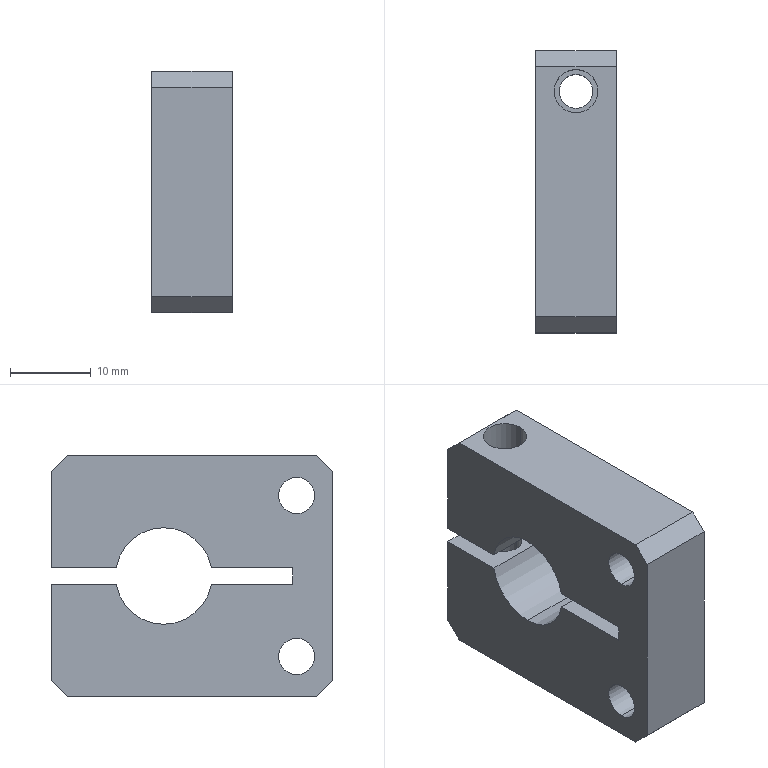Part | STEP file | 11-FG-S02211 | 1 solid | 33 faces | box 10 x 35 x 30 mm | volume 7793 mm3 | plane 18 | cylinder 15 | commonest cylinder face diameters 4.5 x4 8 x4 12 x3 4.2 x2 5.4 x2
STEP:
#1=CARTESIAN_POINT('',(0.6,-13.,-6.));
#2=VERTEX_POINT('',#1);
#3=CARTESIAN_POINT('',(0.6,-13.,-14.));
#4=VERTEX_POINT('',#3);
#5=CARTESIAN_POINT('',(0.6,-13.,-10.));
#6=DIRECTION('',(1.,0.,0.));
#7=DIRECTION('',(0.,0.,-1.));
#8=AXIS2_PLACEMENT_3D('',#5,#6,#7);
#9=CIRCLE('',#8,4.);
#10=EDGE_CURVE('',#2,#4,#9,.T.);
#11=ORIENTED_EDGE('',*,*,#10,.F.);
#12=CARTESIAN_POINT('',(5.,-13.,-6.));
#13=VERTEX_POINT('',#12);
#14=CARTESIAN_POINT('',(5.,-13.,-6.));
#15=DIRECTION('',(1.,0.,0.));
#16=VECTOR('',#15,1000.);
#17=LINE('',#14,#16);
#18=EDGE_CURVE('',#2,#13,#17,.T.);
#19=ORIENTED_EDGE('',*,*,#18,.T.);
#20=CARTESIAN_POINT('',(5.,-13.,-14.));
#21=VERTEX_POINT('',#20);
#22=CARTESIAN_POINT('',(5.,-13.,-10.));
#23=DIRECTION('',(1.,0.,0.));
#24=DIRECTION('',(0.,0.,-1.));
#25=AXIS2_PLACEMENT_3D('',#22,#23,#24);
#26=CIRCLE('',#25,4.);
#27=EDGE_CURVE('',#13,#21,#26,.T.);
#28=ORIENTED_EDGE('',*,*,#27,.T.);
#29=CARTESIAN_POINT('',(5.,-13.,-14.));
#30=DIRECTION('',(1.,0.,0.));
#31=VECTOR('',#30,1000.);
#32=LINE('',#29,#31);
#33=EDGE_CURVE('',#4,#21,#32,.T.);
#34=ORIENTED_EDGE('',*,*,#33,.F.);
#35=EDGE_LOOP('',(#11,#19,#28,#34));
#36=FACE_OUTER_BOUND('',#35,.T.);
#37=CARTESIAN_POINT('',(5.,-13.,-10.));
#38=DIRECTION('',(1.,0.,0.));
#39=DIRECTION('',(0.,0.,-1.));
#40=AXIS2_PLACEMENT_3D('',#37,#38,#39);
#41=CYLINDRICAL_SURFACE('',#40,4.);
#42=ADVANCED_FACE('',(#36),#41,.F.);
#43=CARTESIAN_POINT('',(-5.,-13.,-7.75));
#44=VERTEX_POINT('',#43);
#45=CARTESIAN_POINT('',(-5.,-13.,-12.25));
#46=VERTEX_POINT('',#45);
#47=CARTESIAN_POINT('',(-5.,-13.,-10.));
#48=DIRECTION('',(1.,0.,0.));
#49=DIRECTION('',(0.,0.,-1.));
#50=AXIS2_PLACEMENT_3D('',#47,#48,#49);
#51=CIRCLE('',#50,2.25);
#52=EDGE_CURVE('',#44,#46,#51,.T.);
#53=ORIENTED_EDGE('',*,*,#52,.F.);
#54=CARTESIAN_POINT('',(0.6,-13.,-7.75));
#55=VERTEX_POINT('',#54);
#56=CARTESIAN_POINT('',(5.,-13.,-7.75));
#57=DIRECTION('',(1.,0.,0.));
#58=VECTOR('',#57,1000.);
#59=LINE('',#56,#58);
#60=EDGE_CURVE('',#44,#55,#59,.T.);
#61=ORIENTED_EDGE('',*,*,#60,.T.);
#62=CARTESIAN_POINT('',(0.6,-13.,-12.25));
#63=VERTEX_POINT('',#62);
#64=CARTESIAN_POINT('',(0.6,-13.,-10.));
#65=DIRECTION('',(1.,0.,0.));
#66=DIRECTION('',(0.,0.,-1.));
#67=AXIS2_PLACEMENT_3D('',#64,#65,#66);
#68=CIRCLE('',#67,2.25);
#69=EDGE_CURVE('',#55,#63,#68,.T.);
#70=ORIENTED_EDGE('',*,*,#69,.T.);
#71=CARTESIAN_POINT('',(5.,-13.,-12.25));
#72=DIRECTION('',(1.,0.,0.));
#73=VECTOR('',#72,1000.);
#74=LINE('',#71,#73);
#75=EDGE_CURVE('',#46,#63,#74,.T.);
#76=ORIENTED_EDGE('',*,*,#75,.F.);
#77=EDGE_LOOP('',(#53,#61,#70,#76));
#78=FACE_OUTER_BOUND('',#77,.T.);
#79=CARTESIAN_POINT('',(5.,-13.,-10.));
#80=DIRECTION('',(1.,0.,0.));
#81=DIRECTION('',(0.,0.,-1.));
#82=AXIS2_PLACEMENT_3D('',#79,#80,#81);
#83=CYLINDRICAL_SURFACE('',#82,2.25);
#84=ADVANCED_FACE('',(#78),#83,.F.);
#85=CARTESIAN_POINT('',(0.6,-13.,14.));
#86=VERTEX_POINT('',#85);
#87=CARTESIAN_POINT('',(0.6,-13.,6.));
#88=VERTEX_POINT('',#87);
#89=CARTESIAN_POINT('',(0.6,-13.,10.));
#90=DIRECTION('',(1.,0.,0.));
#91=DIRECTION('',(0.,0.,-1.));
#92=AXIS2_PLACEMENT_3D('',#89,#90,#91);
#93=CIRCLE('',#92,4.);
#94=EDGE_CURVE('',#86,#88,#93,.T.);
#95=ORIENTED_EDGE('',*,*,#94,.F.);
#96=CARTESIAN_POINT('',(5.,-13.,14.));
#97=VERTEX_POINT('',#96);
#98=CARTESIAN_POINT('',(5.,-13.,14.));
#99=DIRECTION('',(1.,0.,0.));
#100=VECTOR('',#99,1000.);
#101=LINE('',#98,#100);
#102=EDGE_CURVE('',#86,#97,#101,.T.);
#103=ORIENTED_EDGE('',*,*,#102,.T.);
#104=CARTESIAN_POINT('',(5.,-13.,6.));
#105=VERTEX_POINT('',#104);
#106=CARTESIAN_POINT('',(5.,-13.,10.));
#107=DIRECTION('',(1.,0.,0.));
#108=DIRECTION('',(0.,0.,-1.));
#109=AXIS2_PLACEMENT_3D('',#106,#107,#108);
#110=CIRCLE('',#109,4.);
#111=EDGE_CURVE('',#97,#105,#110,.T.);
#112=ORIENTED_EDGE('',*,*,#111,.T.);
#113=CARTESIAN_POINT('',(5.,-13.,6.));
#114=DIRECTION('',(1.,0.,0.));
#115=VECTOR('',#114,1000.);
#116=LINE('',#113,#115);
#117=EDGE_CURVE('',#88,#105,#116,.T.);
#118=ORIENTED_EDGE('',*,*,#117,.F.);
#119=EDGE_LOOP('',(#95,#103,#112,#118));
#120=FACE_OUTER_BOUND('',#119,.T.);
#121=CARTESIAN_POINT('',(5.,-13.,10.));
#122=DIRECTION('',(1.,0.,0.));
#123=DIRECTION('',(0.,0.,-1.));
#124=AXIS2_PLACEMENT_3D('',#121,#122,#123);
#125=CYLINDRICAL_SURFACE('',#124,4.);
#126=ADVANCED_FACE('',(#120),#125,.F.);
#127=CARTESIAN_POINT('',(-5.,-13.,12.25));
#128=VERTEX_POINT('',#127);
#129=CARTESIAN_POINT('',(-5.,-13.,7.75));
#130=VERTEX_POINT('',#129);
#131=CARTESIAN_POINT('',(-5.,-13.,10.));
#132=DIRECTION('',(1.,0.,0.));
#133=DIRECTION('',(0.,0.,-1.));
#134=AXIS2_PLACEMENT_3D('',#131,#132,#133);
#135=CIRCLE('',#134,2.25);
#136=EDGE_CURVE('',#128,#130,#135,.T.);
#137=ORIENTED_EDGE('',*,*,#136,.F.);
#138=CARTESIAN_POINT('',(0.6,-13.,12.25));
#139=VERTEX_POINT('',#138);
#140=CARTESIAN_POINT('',(5.,-13.,12.25));
#141=DIRECTION('',(1.,0.,0.));
#142=VECTOR('',#141,1000.);
#143=LINE('',#140,#142);
#144=EDGE_CURVE('',#128,#139,#143,.T.);
#145=ORIENTED_EDGE('',*,*,#144,.T.);
#146=CARTESIAN_POINT('',(0.6,-13.,7.75));
#147=VERTEX_POINT('',#146);
#148=CARTESIAN_POINT('',(0.6,-13.,10.));
#149=DIRECTION('',(1.,0.,0.));
#150=DIRECTION('',(0.,0.,-1.));
#151=AXIS2_PLACEMENT_3D('',#148,#149,#150);
#152=CIRCLE('',#151,2.25);
#153=EDGE_CURVE('',#139,#147,#152,.T.);
#154=ORIENTED_EDGE('',*,*,#153,.T.);
#155=CARTESIAN_POINT('',(5.,-13.,7.75));
#156=DIRECTION('',(1.,0.,0.));
#157=VECTOR('',#156,1000.);
#158=LINE('',#155,#157);
#159=EDGE_CURVE('',#130,#147,#158,.T.);
#160=ORIENTED_EDGE('',*,*,#159,.F.);
#161=EDGE_LOOP('',(#137,#145,#154,#160));
#162=FACE_OUTER_BOUND('',#161,.T.);
#163=CARTESIAN_POINT('',(5.,-13.,10.));
#164=DIRECTION('',(1.,0.,0.));
#165=DIRECTION('',(0.,0.,-1.));
#166=AXIS2_PLACEMENT_3D('',#163,#164,#165);
#167=CYLINDRICAL_SURFACE('',#166,2.25);
#168=ADVANCED_FACE('',(#162),#167,.F.);
#169=CARTESIAN_POINT('',(2.1,12.5,-15.));
#170=VERTEX_POINT('',#169);
#171=CARTESIAN_POINT('',(-2.1,12.5,-15.));
#172=VERTEX_POINT('',#171);
#173=CARTESIAN_POINT('',(0.,12.5,-15.));
#174=DIRECTION('',(0.,0.,-1.));
#175=DIRECTION('',(-1.,0.,0.));
#176=AXIS2_PLACEMENT_3D('',#173,#174,#175);
#177=CIRCLE('',#176,2.1);
#178=EDGE_CURVE('',#170,#172,#177,.T.);
#179=ORIENTED_EDGE('',*,*,#178,.T.);
#180=CARTESIAN_POINT('',(-2.1,12.5,-1.));
#181=VERTEX_POINT('',#180);
#182=CARTESIAN_POINT('',(-2.1,12.5,-1.));
#183=DIRECTION('',(0.,0.,1.));
#184=VECTOR('',#183,1000.);
#185=LINE('',#182,#184);
#186=EDGE_CURVE('',#172,#181,#185,.T.);
#187=ORIENTED_EDGE('',*,*,#186,.T.);
#188=CARTESIAN_POINT('',(2.1,12.5,-1.));
#189=VERTEX_POINT('',#188);
#190=CARTESIAN_POINT('',(0.,12.5,-1.));
#191=DIRECTION('',(0.,0.,1.));
#192=DIRECTION('',(1.,0.,0.));
#193=AXIS2_PLACEMENT_3D('',#190,#191,#192);
#194=CIRCLE('',#193,2.1);
#195=EDGE_CURVE('',#181,#189,#194,.T.);
#196=ORIENTED_EDGE('',*,*,#195,.T.);
#197=CARTESIAN_POINT('',(2.1,12.5,-1.));
#198=DIRECTION('',(0.,0.,1.));
#199=VECTOR('',#198,1000.);
#200=LINE('',#197,#199);
#201=EDGE_CURVE('',#170,#189,#200,.T.);
#202=ORIENTED_EDGE('',*,*,#201,.F.);
#203=EDGE_LOOP('',(#179,#187,#196,#202));
#204=FACE_OUTER_BOUND('',#203,.T.);
#205=CARTESIAN_POINT('',(0.,12.5,-1.));
#206=DIRECTION('',(0.,0.,1.));
#207=DIRECTION('',(1.,0.,0.));
#208=AXIS2_PLACEMENT_3D('',#205,#206,#207);
#209=CYLINDRICAL_SURFACE('',#208,2.1);
#210=ADVANCED_FACE('',(#204),#209,.F.);
#211=CARTESIAN_POINT('',(-2.7,12.5,1.));
#212=VERTEX_POINT('',#211);
#213=CARTESIAN_POINT('',(2.7,12.5,1.));
#214=VERTEX_POINT('',#213);
#215=CARTESIAN_POINT('',(0.,12.5,1.));
#216=DIRECTION('',(0.,0.,1.));
#217=DIRECTION('',(0.,-1.,0.));
#218=AXIS2_PLACEMENT_3D('',#215,#216,#217);
#219=CIRCLE('',#218,2.7);
#220=EDGE_CURVE('',#212,#214,#219,.T.);
#221=ORIENTED_EDGE('',*,*,#220,.F.);
#222=CARTESIAN_POINT('',(-2.7,12.5,15.));
#223=VERTEX_POINT('',#222);
#224=CARTESIAN_POINT('',(-2.7,12.5,15.));
#225=DIRECTION('',(0.,0.,1.));
#226=VECTOR('',#225,1000.);
#227=LINE('',#224,#226);
#228=EDGE_CURVE('',#212,#223,#227,.T.);
#229=ORIENTED_EDGE('',*,*,#228,.T.);
#230=CARTESIAN_POINT('',(2.7,12.5,15.));
#231=VERTEX_POINT('',#230);
#232=CARTESIAN_POINT('',(0.,12.5,15.));
#233=DIRECTION('',(0.,0.,1.));
#234=DIRECTION('',(1.,0.,0.));
#235=AXIS2_PLACEMENT_3D('',#232,#233,#234);
#236=CIRCLE('',#235,2.7);
#237=EDGE_CURVE('',#223,#231,#236,.T.);
#238=ORIENTED_EDGE('',*,*,#237,.T.);
#239=CARTESIAN_POINT('',(2.7,12.5,15.));
#240=DIRECTION('',(0.,0.,1.));
#241=VECTOR('',#240,1000.);
#242=LINE('',#239,#241);
#243=EDGE_CURVE('',#214,#231,#242,.T.);
#244=ORIENTED_EDGE('',*,*,#243,.F.);
#245=EDGE_LOOP('',(#221,#229,#238,#244));
#246=FACE_OUTER_BOUND('',#245,.T.);
#247=CARTESIAN_POINT('',(0.,12.5,15.));
#248=DIRECTION('',(0.,0.,1.));
#249=DIRECTION('',(1.,0.,0.));
#250=AXIS2_PLACEMENT_3D('',#247,#248,#249);
#251=CYLINDRICAL_SURFACE('',#250,2.7);
#252=ADVANCED_FACE('',(#246),#251,.F.);
#253=CARTESIAN_POINT('',(-5.,3.5,-6.));
#254=VERTEX_POINT('',#253);
#255=CARTESIAN_POINT('',(-5.,9.416,-1.));
#256=VERTEX_POINT('',#255);
#257=CARTESIAN_POINT('',(-5.,3.5,0.));
#258=DIRECTION('',(1.,0.,0.));
#259=DIRECTION('',(0.,0.,-1.));
#260=AXIS2_PLACEMENT_3D('',#257,#258,#259);
#261=CIRCLE('',#260,6.);
#262=EDGE_CURVE('',#254,#256,#261,.T.);
#263=ORIENTED_EDGE('',*,*,#262,.F.);
#264=CARTESIAN_POINT('',(5.,3.5,-6.));
#265=VERTEX_POINT('',#264);
#266=CARTESIAN_POINT('',(-5.,3.5,-6.));
#267=DIRECTION('',(1.,0.,0.));
#268=VECTOR('',#267,1000.);
#269=LINE('',#266,#268);
#270=EDGE_CURVE('',#254,#265,#269,.T.);
#271=ORIENTED_EDGE('',*,*,#270,.T.);
#272=CARTESIAN_POINT('',(5.,9.416,-1.));
#273=VERTEX_POINT('',#272);
#274=CARTESIAN_POINT('',(5.,3.5,0.));
#275=DIRECTION('',(1.,0.,0.));
#276=DIRECTION('',(0.,0.,-1.));
#277=AXIS2_PLACEMENT_3D('',#274,#275,#276);
#278=CIRCLE('',#277,6.);
#279=EDGE_CURVE('',#265,#273,#278,.T.);
#280=ORIENTED_EDGE('',*,*,#279,.T.);
#281=CARTESIAN_POINT('',(-5.,9.416,-1.));
#282=DIRECTION('',(-1.,0.,0.));
#283=VECTOR('',#282,1000.);
#284=LINE('',#281,#283);
#285=EDGE_CURVE('',#273,#256,#284,.T.);
#286=ORIENTED_EDGE('',*,*,#285,.T.);
#287=EDGE_LOOP('',(#263,#271,#280,#286));
#288=FACE_OUTER_BOUND('',#287,.T.);
#289=CARTESIAN_POINT('',(-5.,3.5,0.));
#290=DIRECTION('',(1.,0.,0.));
#291=DIRECTION('',(0.,0.,-1.));
#292=AXIS2_PLACEMENT_3D('',#289,#290,#291);
#293=CYLINDRICAL_SURFACE('',#292,6.);
#294=ADVANCED_FACE('',(#288),#293,.F.);
#295=CARTESIAN_POINT('',(5.,17.5,-1.));
#296=VERTEX_POINT('',#295);
#297=CARTESIAN_POINT('',(5.,17.5,-1.));
#298=DIRECTION('',(0.,1.,0.));
#299=VECTOR('',#298,1000.);
#300=LINE('',#297,#299);
#301=EDGE_CURVE('',#273,#296,#300,.T.);
#302=ORIENTED_EDGE('',*,*,#301,.T.);
#303=CARTESIAN_POINT('',(-5.,17.5,-1.));
#304=VERTEX_POINT('',#303);
#305=CARTESIAN_POINT('',(-5.,17.5,-1.));
#306=DIRECTION('',(1.,0.,0.));
#307=VECTOR('',#306,1000.);
#308=LINE('',#305,#307);
#309=EDGE_CURVE('',#304,#296,#308,.T.);
#310=ORIENTED_EDGE('',*,*,#309,.F.);
#311=CARTESIAN_POINT('',(-5.,17.5,-1.));
#312=DIRECTION('',(0.,1.,0.));
#313=VECTOR('',#312,1000.);
#314=LINE('',#311,#313);
#315=EDGE_CURVE('',#256,#304,#314,.T.);
#316=ORIENTED_EDGE('',*,*,#315,.F.);
#317=ORIENTED_EDGE('',*,*,#285,.F.);
#318=EDGE_LOOP('',(#302,#310,#316,#317));
#319=FACE_OUTER_BOUND('',#318,.T.);
#320=CARTESIAN_POINT('',(0.,12.5,-1.));
#321=DIRECTION('',(0.,0.,1.));
#322=DIRECTION('',(1.,0.,0.));
#323=AXIS2_PLACEMENT_3D('',#320,#321,#322);
#324=CIRCLE('',#323,2.1);
#325=EDGE_CURVE('',#189,#181,#324,.T.);
#326=ORIENTED_EDGE('',*,*,#325,.F.);
#327=ORIENTED_EDGE('',*,*,#195,.F.);
#328=EDGE_LOOP('',(#326,#327));
#329=FACE_BOUND('',#328,.T.);
#330=CARTESIAN_POINT('',(-5.,17.5,-1.));
#331=DIRECTION('',(0.,0.,-1.));
#332=DIRECTION('',(0.,1.,0.));
#333=AXIS2_PLACEMENT_3D('',#330,#331,#332);
#334=PLANE('',#333);
#335=ADVANCED_FACE('',(#319,#329),#334,.F.);
#336=CARTESIAN_POINT('',(5.,-15.5,15.));
#337=VERTEX_POINT('',#336);
#338=CARTESIAN_POINT('',(5.,15.5,15.));
#339=VERTEX_POINT('',#338);
#340=CARTESIAN_POINT('',(5.,-17.5,15.));
#341=DIRECTION('',(0.,1.,0.));
#342=VECTOR('',#341,1000.);
#343=LINE('',#340,#342);
#344=EDGE_CURVE('',#337,#339,#343,.T.);
#345=ORIENTED_EDGE('',*,*,#344,.T.);
#346=CARTESIAN_POINT('',(-5.,15.5,15.));
#347=VERTEX_POINT('',#346);
#348=CARTESIAN_POINT('',(0.,15.5,15.));
#349=DIRECTION('',(-1.,0.,0.));
#350=VECTOR('',#349,1000.);
#351=LINE('',#348,#350);
#352=EDGE_CURVE('',#339,#347,#351,.T.);
#353=ORIENTED_EDGE('',*,*,#352,.T.);
#354=CARTESIAN_POINT('',(-5.,-15.5,15.));
#355=VERTEX_POINT('',#354);
#356=CARTESIAN_POINT('',(-5.,-17.5,15.));
#357=DIRECTION('',(0.,-1.,0.));
#358=VECTOR('',#357,1000.);
#359=LINE('',#356,#358);
#360=EDGE_CURVE('',#347,#355,#359,.T.);
#361=ORIENTED_EDGE('',*,*,#360,.T.);
#362=CARTESIAN_POINT('',(0.,-15.5,15.));
#363=DIRECTION('',(1.,0.,0.));
#364=VECTOR('',#363,1000.);
#365=LINE('',#362,#364);
#366=EDGE_CURVE('',#355,#337,#365,.T.);
#367=ORIENTED_EDGE('',*,*,#366,.T.);
#368=EDGE_LOOP('',(#345,#353,#361,#367));
#369=FACE_OUTER_BOUND('',#368,.T.);
#370=CARTESIAN_POINT('',(0.,12.5,15.));
#371=DIRECTION('',(0.,0.,1.));
#372=DIRECTION('',(1.,0.,0.));
#373=AXIS2_PLACEMENT_3D('',#370,#371,#372);
#374=CIRCLE('',#373,2.7);
#375=EDGE_CURVE('',#231,#223,#374,.T.);
#376=ORIENTED_EDGE('',*,*,#375,.F.);
#377=ORIENTED_EDGE('',*,*,#237,.F.);
#378=EDGE_LOOP('',(#376,#377));
#379=FACE_BOUND('',#378,.T.);
#380=CARTESIAN_POINT('',(0.,0.,15.));
#381=DIRECTION('',(0.,0.,-1.));
#382=DIRECTION('',(-1.,0.,0.));
#383=AXIS2_PLACEMENT_3D('',#380,#381,#382);
#384=PLANE('',#383);
#385=ADVANCED_FACE('',(#369,#379),#384,.F.);
#386=CARTESIAN_POINT('',(-5.,17.5,13.));
#387=VERTEX_POINT('',#386);
#388=CARTESIAN_POINT('',(-5.,17.5,1.));
#389=VERTEX_POINT('',#388);
#390=CARTESIAN_POINT('',(-5.,17.5,15.));
#391=DIRECTION('',(0.,0.,-1.));
#392=VECTOR('',#391,1000.);
#393=LINE('',#390,#392);
#394=EDGE_CURVE('',#387,#389,#393,.T.);
#395=ORIENTED_EDGE('',*,*,#394,.F.);
#396=CARTESIAN_POINT('',(5.,17.5,13.));
#397=VERTEX_POINT('',#396);
#398=CARTESIAN_POINT('',(-5.,17.5,13.));
#399=DIRECTION('',(1.,0.,0.));
#400=VECTOR('',#399,1000.);
#401=LINE('',#398,#400);
#402=EDGE_CURVE('',#387,#397,#401,.T.);
#403=ORIENTED_EDGE('',*,*,#402,.T.);
#404=CARTESIAN_POINT('',(5.,17.5,1.));
#405=VERTEX_POINT('',#404);
#406=CARTESIAN_POINT('',(5.,17.5,15.));
#407=DIRECTION('',(0.,0.,-1.));
#408=VECTOR('',#407,1000.);
#409=LINE('',#406,#408);
#410=EDGE_CURVE('',#397,#405,#409,.T.);
#411=ORIENTED_EDGE('',*,*,#410,.T.);
#412=CARTESIAN_POINT('',(-5.,17.5,1.));
#413=DIRECTION('',(1.,0.,0.));
#414=VECTOR('',#413,1000.);
#415=LINE('',#412,#414);
#416=EDGE_CURVE('',#389,#405,#415,.T.);
#417=ORIENTED_EDGE('',*,*,#416,.F.);
#418=EDGE_LOOP('',(#395,#403,#411,#417));
#419=FACE_OUTER_BOUND('',#418,.T.);
#420=CARTESIAN_POINT('',(-5.,17.5,15.));
#421=DIRECTION('',(0.,-1.,0.));
#422=DIRECTION('',(0.,0.,-1.));
#423=AXIS2_PLACEMENT_3D('',#420,#421,#422);
#424=PLANE('',#423);
#425=ADVANCED_FACE('',(#419),#424,.F.);
#426=CARTESIAN_POINT('',(5.,9.416,1.));
#427=VERTEX_POINT('',#426);
#428=CARTESIAN_POINT('',(5.,-2.416,1.));
#429=VERTEX_POINT('',#428);
#430=CARTESIAN_POINT('',(5.,3.5,0.));
#431=DIRECTION('',(1.,0.,0.));
#432=DIRECTION('',(0.,0.,-1.));
#433=AXIS2_PLACEMENT_3D('',#430,#431,#432);
#434=CIRCLE('',#433,6.);
#435=EDGE_CURVE('',#427,#429,#434,.T.);
#436=ORIENTED_EDGE('',*,*,#435,.T.);
#437=CARTESIAN_POINT('',(-5.,-2.416,1.));
#438=VERTEX_POINT('',#437);
#439=CARTESIAN_POINT('',(-5.,-2.416,1.));
#440=DIRECTION('',(-1.,0.,0.));
#441=VECTOR('',#440,1000.);
#442=LINE('',#439,#441);
#443=EDGE_CURVE('',#429,#438,#442,.T.);
#444=ORIENTED_EDGE('',*,*,#443,.T.);
#445=CARTESIAN_POINT('',(-5.,9.416,1.));
#446=VERTEX_POINT('',#445);
#447=CARTESIAN_POINT('',(-5.,3.5,0.));
#448=DIRECTION('',(1.,0.,0.));
#449=DIRECTION('',(0.,0.,-1.));
#450=AXIS2_PLACEMENT_3D('',#447,#448,#449);
#451=CIRCLE('',#450,6.);
#452=EDGE_CURVE('',#446,#438,#451,.T.);
#453=ORIENTED_EDGE('',*,*,#452,.F.);
#454=CARTESIAN_POINT('',(-5.,9.416,1.));
#455=DIRECTION('',(1.,0.,0.));
#456=VECTOR('',#455,1000.);
#457=LINE('',#454,#456);
#458=EDGE_CURVE('',#446,#427,#457,.T.);
#459=ORIENTED_EDGE('',*,*,#458,.T.);
#460=EDGE_LOOP('',(#436,#444,#453,#459));
#461=FACE_OUTER_BOUND('',#460,.T.);
#462=CARTESIAN_POINT('',(-5.,3.5,0.));
#463=DIRECTION('',(1.,0.,0.));
#464=DIRECTION('',(0.,0.,-1.));
#465=AXIS2_PLACEMENT_3D('',#462,#463,#464);
#466=CYLINDRICAL_SURFACE('',#465,6.);
#467=ADVANCED_FACE('',(#461),#466,.F.);
#468=CARTESIAN_POINT('',(5.,-13.,-10.));
#469=DIRECTION('',(1.,0.,0.));
#470=DIRECTION('',(0.,0.,-1.));
#471=AXIS2_PLACEMENT_3D('',#468,#469,#470);
#472=CIRCLE('',#471,4.);
#473=EDGE_CURVE('',#21,#13,#472,.T.);
#474=ORIENTED_EDGE('',*,*,#473,.F.);
#475=ORIENTED_EDGE('',*,*,#27,.F.);
#476=EDGE_LOOP('',(#474,#475));
#477=FACE_BOUND('',#476,.T.);
#478=CARTESIAN_POINT('',(5.,-13.,10.));
#479=DIRECTION('',(1.,0.,0.));
#480=DIRECTION('',(0.,0.,-1.));
#481=AXIS2_PLACEMENT_3D('',#478,#479,#480);
#482=CIRCLE('',#481,4.);
#483=EDGE_CURVE('',#105,#97,#482,.T.);
#484=ORIENTED_EDGE('',*,*,#483,.F.);
#485=ORIENTED_EDGE('',*,*,#111,.F.);
#486=EDGE_LOOP('',(#484,#485));
#487=FACE_BOUND('',#486,.T.);
#488=CARTESIAN_POINT('',(5.,-15.5,-15.));
#489=VERTEX_POINT('',#488);
#490=CARTESIAN_POINT('',(5.,15.5,-15.));
#491=VERTEX_POINT('',#490);
#492=CARTESIAN_POINT('',(5.,-17.5,-15.));
#493=DIRECTION('',(0.,1.,0.));
#494=VECTOR('',#493,1000.);
#495=LINE('',#492,#494);
#496=EDGE_CURVE('',#489,#491,#495,.T.);
#497=ORIENTED_EDGE('',*,*,#496,.T.);
#498=CARTESIAN_POINT('',(5.,17.5,-13.));
#499=VERTEX_POINT('',#498);
#500=CARTESIAN_POINT('',(5.,17.5,-13.));
#501=DIRECTION('',(0.,0.7071,0.7071));
#502=VECTOR('',#501,1000.);
#503=LINE('',#500,#502);
#504=EDGE_CURVE('',#491,#499,#503,.T.);
#505=ORIENTED_EDGE('',*,*,#504,.T.);
#506=CARTESIAN_POINT('',(5.,17.5,15.));
#507=DIRECTION('',(0.,0.,-1.));
#508=VECTOR('',#507,1000.);
#509=LINE('',#506,#508);
#510=EDGE_CURVE('',#296,#499,#509,.T.);
#511=ORIENTED_EDGE('',*,*,#510,.F.);
#512=ORIENTED_EDGE('',*,*,#301,.F.);
#513=ORIENTED_EDGE('',*,*,#279,.F.);
#514=CARTESIAN_POINT('',(5.,-2.416,-1.));
#515=VERTEX_POINT('',#514);
#516=CARTESIAN_POINT('',(5.,3.5,0.));
#517=DIRECTION('',(1.,0.,0.));
#518=DIRECTION('',(0.,0.,-1.));
#519=AXIS2_PLACEMENT_3D('',#516,#517,#518);
#520=CIRCLE('',#519,6.);
#521=EDGE_CURVE('',#515,#265,#520,.T.);
#522=ORIENTED_EDGE('',*,*,#521,.F.);
#523=CARTESIAN_POINT('',(5.,-12.5,-1.));
#524=VERTEX_POINT('',#523);
#525=CARTESIAN_POINT('',(5.,17.5,-1.));
#526=DIRECTION('',(0.,1.,0.));
#527=VECTOR('',#526,1000.);
#528=LINE('',#525,#527);
#529=EDGE_CURVE('',#524,#515,#528,.T.);
#530=ORIENTED_EDGE('',*,*,#529,.F.);
#531=CARTESIAN_POINT('',(5.,-12.5,1.));
#532=VERTEX_POINT('',#531);
#533=CARTESIAN_POINT('',(5.,-12.5,1.));
#534=DIRECTION('',(0.,0.,-1.));
#535=VECTOR('',#534,1000.);
#536=LINE('',#533,#535);
#537=EDGE_CURVE('',#532,#524,#536,.T.);
#538=ORIENTED_EDGE('',*,*,#537,.F.);
#539=CARTESIAN_POINT('',(5.,17.5,1.));
#540=DIRECTION('',(0.,-1.,0.));
#541=VECTOR('',#540,1000.);
#542=LINE('',#539,#541);
#543=EDGE_CURVE('',#429,#532,#542,.T.);
#544=ORIENTED_EDGE('',*,*,#543,.F.);
#545=ORIENTED_EDGE('',*,*,#435,.F.);
#546=CARTESIAN_POINT('',(5.,17.5,1.));
#547=DIRECTION('',(0.,-1.,0.));
#548=VECTOR('',#547,1000.);
#549=LINE('',#546,#548);
#550=EDGE_CURVE('',#405,#427,#549,.T.);
#551=ORIENTED_EDGE('',*,*,#550,.F.);
#552=ORIENTED_EDGE('',*,*,#410,.F.);
#553=CARTESIAN_POINT('',(5.,15.5,15.));
#554=DIRECTION('',(0.,-0.7071,0.7071));
#555=VECTOR('',#554,1000.);
#556=LINE('',#553,#555);
#557=EDGE_CURVE('',#397,#339,#556,.T.);
#558=ORIENTED_EDGE('',*,*,#557,.T.);
#559=ORIENTED_EDGE('',*,*,#344,.F.);
#560=CARTESIAN_POINT('',(5.,-17.5,13.));
#561=VERTEX_POINT('',#560);
#562=CARTESIAN_POINT('',(5.,-15.5,15.));
#563=DIRECTION('',(0.,-0.7071,-0.7071));
#564=VECTOR('',#563,1000.);
#565=LINE('',#562,#564);
#566=EDGE_CURVE('',#337,#561,#565,.T.);
#567=ORIENTED_EDGE('',*,*,#566,.T.);
#568=CARTESIAN_POINT('',(5.,-17.5,-13.));
#569=VERTEX_POINT('',#568);
#570=CARTESIAN_POINT('',(5.,-17.5,15.));
#571=DIRECTION('',(0.,0.,-1.));
#572=VECTOR('',#571,1000.);
#573=LINE('',#570,#572);
#574=EDGE_CURVE('',#561,#569,#573,.T.);
#575=ORIENTED_EDGE('',*,*,#574,.T.);
#576=CARTESIAN_POINT('',(5.,-17.5,-13.));
#577=DIRECTION('',(0.,0.7071,-0.7071));
#578=VECTOR('',#577,1000.);
#579=LINE('',#576,#578);
#580=EDGE_CURVE('',#569,#489,#579,.T.);
#581=ORIENTED_EDGE('',*,*,#580,.T.);
#582=EDGE_LOOP('',(#497,#505,#511,#512,#513,#522,#530,#538,#544,#545,#551,#552,#558,#559,#567,#575,#581));
#583=FACE_OUTER_BOUND('',#582,.T.);
#584=CARTESIAN_POINT('',(5.,-17.5,15.));
#585=DIRECTION('',(-1.,0.,0.));
#586=DIRECTION('',(0.,0.,1.));
#587=AXIS2_PLACEMENT_3D('',#584,#585,#586);
#588=PLANE('',#587);
#589=ADVANCED_FACE('',(#477,#487,#583),#588,.F.);
#590=ORIENTED_EDGE('',*,*,#510,.T.);
#591=CARTESIAN_POINT('',(-5.,17.5,-13.));
#592=VERTEX_POINT('',#591);
#593=CARTESIAN_POINT('',(-5.,17.5,-13.));
#594=DIRECTION('',(-1.,0.,0.));
#595=VECTOR('',#594,1000.);
#596=LINE('',#593,#595);
#597=EDGE_CURVE('',#499,#592,#596,.T.);
#598=ORIENTED_EDGE('',*,*,#597,.T.);
#599=CARTESIAN_POINT('',(-5.,17.5,15.));
#600=DIRECTION('',(0.,0.,-1.));
#601=VECTOR('',#600,1000.);
#602=LINE('',#599,#601);
#603=EDGE_CURVE('',#304,#592,#602,.T.);
#604=ORIENTED_EDGE('',*,*,#603,.F.);
#605=ORIENTED_EDGE('',*,*,#309,.T.);
#606=EDGE_LOOP('',(#590,#598,#604,#605));
#607=FACE_OUTER_BOUND('',#606,.T.);
#608=CARTESIAN_POINT('',(-5.,17.5,15.));
#609=DIRECTION('',(0.,-1.,0.));
#610=DIRECTION('',(0.,0.,-1.));
#611=AXIS2_PLACEMENT_3D('',#608,#609,#610);
#612=PLANE('',#611);
#613=ADVANCED_FACE('',(#607),#612,.F.);
#614=CARTESIAN_POINT('',(-5.,-13.,-10.));
#615=DIRECTION('',(1.,0.,0.));
#616=DIRECTION('',(0.,0.,-1.));
#617=AXIS2_PLACEMENT_3D('',#614,#615,#616);
#618=CIRCLE('',#617,2.25);
#619=EDGE_CURVE('',#46,#44,#618,.T.);
#620=ORIENTED_EDGE('',*,*,#619,.T.);
#621=ORIENTED_EDGE('',*,*,#52,.T.);
#622=EDGE_LOOP('',(#620,#621));
#623=FACE_BOUND('',#622,.T.);
#624=CARTESIAN_POINT('',(-5.,-13.,10.));
#625=DIRECTION('',(1.,0.,0.));
#626=DIRECTION('',(0.,0.,-1.));
#627=AXIS2_PLACEMENT_3D('',#624,#625,#626);
#628=CIRCLE('',#627,2.25);
#629=EDGE_CURVE('',#130,#128,#628,.T.);
#630=ORIENTED_EDGE('',*,*,#629,.T.);
#631=ORIENTED_EDGE('',*,*,#136,.T.);
#632=EDGE_LOOP('',(#630,#631));
#633=FACE_BOUND('',#632,.T.);
#634=ORIENTED_EDGE('',*,*,#603,.T.);
#635=CARTESIAN_POINT('',(-5.,15.5,-15.));
#636=VERTEX_POINT('',#635);
#637=CARTESIAN_POINT('',(-5.,17.5,-13.));
#638=DIRECTION('',(0.,-0.7071,-0.7071));
#639=VECTOR('',#638,1000.);
#640=LINE('',#637,#639);
#641=EDGE_CURVE('',#592,#636,#640,.T.);
#642=ORIENTED_EDGE('',*,*,#641,.T.);
#643=CARTESIAN_POINT('',(-5.,-15.5,-15.));
#644=VERTEX_POINT('',#643);
#645=CARTESIAN_POINT('',(-5.,-17.5,-15.));
#646=DIRECTION('',(0.,-1.,0.));
#647=VECTOR('',#646,1000.);
#648=LINE('',#645,#647);
#649=EDGE_CURVE('',#636,#644,#648,.T.);
#650=ORIENTED_EDGE('',*,*,#649,.T.);
#651=CARTESIAN_POINT('',(-5.,-17.5,-13.));
#652=VERTEX_POINT('',#651);
#653=CARTESIAN_POINT('',(-5.,-17.5,-13.));
#654=DIRECTION('',(0.,-0.7071,0.7071));
#655=VECTOR('',#654,1000.);
#656=LINE('',#653,#655);
#657=EDGE_CURVE('',#644,#652,#656,.T.);
#658=ORIENTED_EDGE('',*,*,#657,.T.);
#659=CARTESIAN_POINT('',(-5.,-17.5,13.));
#660=VERTEX_POINT('',#659);
#661=CARTESIAN_POINT('',(-5.,-17.5,15.));
#662=DIRECTION('',(0.,0.,-1.));
#663=VECTOR('',#662,1000.);
#664=LINE('',#661,#663);
#665=EDGE_CURVE('',#660,#652,#664,.T.);
#666=ORIENTED_EDGE('',*,*,#665,.F.);
#667=CARTESIAN_POINT('',(-5.,-15.5,15.));
#668=DIRECTION('',(0.,0.7071,0.7071));
#669=VECTOR('',#668,1000.);
#670=LINE('',#667,#669);
#671=EDGE_CURVE('',#660,#355,#670,.T.);
#672=ORIENTED_EDGE('',*,*,#671,.T.);
#673=ORIENTED_EDGE('',*,*,#360,.F.);
#674=CARTESIAN_POINT('',(-5.,15.5,15.));
#675=DIRECTION('',(0.,0.7071,-0.7071));
#676=VECTOR('',#675,1000.);
#677=LINE('',#674,#676);
#678=EDGE_CURVE('',#347,#387,#677,.T.);
#679=ORIENTED_EDGE('',*,*,#678,.T.);
#680=ORIENTED_EDGE('',*,*,#394,.T.);
#681=CARTESIAN_POINT('',(-5.,17.5,1.));
#682=DIRECTION('',(0.,-1.,0.));
#683=VECTOR('',#682,1000.);
#684=LINE('',#681,#683);
#685=EDGE_CURVE('',#389,#446,#684,.T.);
#686=ORIENTED_EDGE('',*,*,#685,.T.);
#687=ORIENTED_EDGE('',*,*,#452,.T.);
#688=CARTESIAN_POINT('',(-5.,-12.5,1.));
#689=VERTEX_POINT('',#688);
#690=CARTESIAN_POINT('',(-5.,17.5,1.));
#691=DIRECTION('',(0.,-1.,0.));
#692=VECTOR('',#691,1000.);
#693=LINE('',#690,#692);
#694=EDGE_CURVE('',#438,#689,#693,.T.);
#695=ORIENTED_EDGE('',*,*,#694,.T.);
#696=CARTESIAN_POINT('',(-5.,-12.5,-1.));
#697=VERTEX_POINT('',#696);
#698=CARTESIAN_POINT('',(-5.,-12.5,1.));
#699=DIRECTION('',(0.,0.,-1.));
#700=VECTOR('',#699,1000.);
#701=LINE('',#698,#700);
#702=EDGE_CURVE('',#689,#697,#701,.T.);
#703=ORIENTED_EDGE('',*,*,#702,.T.);
#704=CARTESIAN_POINT('',(-5.,-2.416,-1.));
#705=VERTEX_POINT('',#704);
#706=CARTESIAN_POINT('',(-5.,17.5,-1.));
#707=DIRECTION('',(0.,1.,0.));
#708=VECTOR('',#707,1000.);
#709=LINE('',#706,#708);
#710=EDGE_CURVE('',#697,#705,#709,.T.);
#711=ORIENTED_EDGE('',*,*,#710,.T.);
#712=CARTESIAN_POINT('',(-5.,3.5,0.));
#713=DIRECTION('',(1.,0.,0.));
#714=DIRECTION('',(0.,0.,-1.));
#715=AXIS2_PLACEMENT_3D('',#712,#713,#714);
#716=CIRCLE('',#715,6.);
#717=EDGE_CURVE('',#705,#254,#716,.T.);
#718=ORIENTED_EDGE('',*,*,#717,.T.);
#719=ORIENTED_EDGE('',*,*,#262,.T.);
#720=ORIENTED_EDGE('',*,*,#315,.T.);
#721=EDGE_LOOP('',(#634,#642,#650,#658,#666,#672,#673,#679,#680,#686,#687,#695,#703,#711,#718,#719,#720));
#722=FACE_OUTER_BOUND('',#721,.T.);
#723=CARTESIAN_POINT('',(-5.,-17.5,15.));
#724=DIRECTION('',(1.,0.,0.));
#725=DIRECTION('',(0.,0.,-1.));
#726=AXIS2_PLACEMENT_3D('',#723,#724,#725);
#727=PLANE('',#726);
#728=ADVANCED_FACE('',(#623,#633,#722),#727,.F.);
#729=ORIENTED_EDGE('',*,*,#574,.F.);
#730=CARTESIAN_POINT('',(-5.,-17.5,13.));
#731=DIRECTION('',(-1.,0.,0.));
#732=VECTOR('',#731,1000.);
#733=LINE('',#730,#732);
#734=EDGE_CURVE('',#561,#660,#733,.T.);
#735=ORIENTED_EDGE('',*,*,#734,.T.);
#736=ORIENTED_EDGE('',*,*,#665,.T.);
#737=CARTESIAN_POINT('',(5.,-17.5,-13.));
#738=DIRECTION('',(1.,0.,0.));
#739=VECTOR('',#738,1000.);
#740=LINE('',#737,#739);
#741=EDGE_CURVE('',#652,#569,#740,.T.);
#742=ORIENTED_EDGE('',*,*,#741,.T.);
#743=EDGE_LOOP('',(#729,#735,#736,#742));
#744=FACE_OUTER_BOUND('',#743,.T.);
#745=CARTESIAN_POINT('',(-5.,-17.5,15.));
#746=DIRECTION('',(0.,1.,0.));
#747=DIRECTION('',(0.,0.,1.));
#748=AXIS2_PLACEMENT_3D('',#745,#746,#747);
#749=PLANE('',#748);
#750=ADVANCED_FACE('',(#744),#749,.F.);
#751=ORIENTED_EDGE('',*,*,#178,.F.);
#752=CARTESIAN_POINT('',(0.,12.5,-15.));
#753=DIRECTION('',(0.,0.,-1.));
#754=DIRECTION('',(-1.,0.,0.));
#755=AXIS2_PLACEMENT_3D('',#752,#753,#754);
#756=CIRCLE('',#755,2.1);
#757=EDGE_CURVE('',#172,#170,#756,.T.);
#758=ORIENTED_EDGE('',*,*,#757,.F.);
#759=EDGE_LOOP('',(#751,#758));
#760=FACE_BOUND('',#759,.T.);
#761=ORIENTED_EDGE('',*,*,#649,.F.);
#762=CARTESIAN_POINT('',(5.,15.5,-15.));
#763=DIRECTION('',(1.,0.,0.));
#764=VECTOR('',#763,1000.);
#765=LINE('',#762,#764);
#766=EDGE_CURVE('',#636,#491,#765,.T.);
#767=ORIENTED_EDGE('',*,*,#766,.T.);
#768=ORIENTED_EDGE('',*,*,#496,.F.);
#769=CARTESIAN_POINT('',(-5.,-15.5,-15.));
#770=DIRECTION('',(-1.,0.,0.));
#771=VECTOR('',#770,1000.);
#772=LINE('',#769,#771);
#773=EDGE_CURVE('',#489,#644,#772,.T.);
#774=ORIENTED_EDGE('',*,*,#773,.T.);
#775=EDGE_LOOP('',(#761,#767,#768,#774));
#776=FACE_OUTER_BOUND('',#775,.T.);
#777=CARTESIAN_POINT('',(0.,0.,-15.));
#778=DIRECTION('',(0.,0.,-1.));
#779=DIRECTION('',(-1.,0.,0.));
#780=AXIS2_PLACEMENT_3D('',#777,#778,#779);
#781=PLANE('',#780);
#782=ADVANCED_FACE('',(#760,#776),#781,.T.);
#783=ORIENTED_EDGE('',*,*,#270,.F.);
#784=ORIENTED_EDGE('',*,*,#717,.F.);
#785=CARTESIAN_POINT('',(-5.,-2.416,-1.));
#786=DIRECTION('',(1.,0.,0.));
#787=VECTOR('',#786,1000.);
#788=LINE('',#785,#787);
#789=EDGE_CURVE('',#705,#515,#788,.T.);
#790=ORIENTED_EDGE('',*,*,#789,.T.);
#791=ORIENTED_EDGE('',*,*,#521,.T.);
#792=EDGE_LOOP('',(#783,#784,#790,#791));
#793=FACE_OUTER_BOUND('',#792,.T.);
#794=CARTESIAN_POINT('',(-5.,3.5,0.));
#795=DIRECTION('',(1.,0.,0.));
#796=DIRECTION('',(0.,0.,-1.));
#797=AXIS2_PLACEMENT_3D('',#794,#795,#796);
#798=CYLINDRICAL_SURFACE('',#797,6.);
#799=ADVANCED_FACE('',(#793),#798,.F.);
#800=ORIENTED_EDGE('',*,*,#710,.F.);
#801=CARTESIAN_POINT('',(-5.,-12.5,-1.));
#802=DIRECTION('',(1.,0.,0.));
#803=VECTOR('',#802,1000.);
#804=LINE('',#801,#803);
#805=EDGE_CURVE('',#697,#524,#804,.T.);
#806=ORIENTED_EDGE('',*,*,#805,.T.);
#807=ORIENTED_EDGE('',*,*,#529,.T.);
#808=ORIENTED_EDGE('',*,*,#789,.F.);
#809=EDGE_LOOP('',(#800,#806,#807,#808));
#810=FACE_OUTER_BOUND('',#809,.T.);
#811=CARTESIAN_POINT('',(-5.,17.5,-1.));
#812=DIRECTION('',(0.,0.,-1.));
#813=DIRECTION('',(0.,1.,0.));
#814=AXIS2_PLACEMENT_3D('',#811,#812,#813);
#815=PLANE('',#814);
#816=ADVANCED_FACE('',(#810),#815,.F.);
#817=ORIENTED_EDGE('',*,*,#543,.T.);
#818=CARTESIAN_POINT('',(-5.,-12.5,1.));
#819=DIRECTION('',(1.,0.,0.));
#820=VECTOR('',#819,1000.);
#821=LINE('',#818,#820);
#822=EDGE_CURVE('',#689,#532,#821,.T.);
#823=ORIENTED_EDGE('',*,*,#822,.F.);
#824=ORIENTED_EDGE('',*,*,#694,.F.);
#825=ORIENTED_EDGE('',*,*,#443,.F.);
#826=EDGE_LOOP('',(#817,#823,#824,#825));
#827=FACE_OUTER_BOUND('',#826,.T.);
#828=CARTESIAN_POINT('',(-5.,17.5,1.));
#829=DIRECTION('',(0.,0.,1.));
#830=DIRECTION('',(0.,-1.,0.));
#831=AXIS2_PLACEMENT_3D('',#828,#829,#830);
#832=PLANE('',#831);
#833=ADVANCED_FACE('',(#827),#832,.F.);
#834=ORIENTED_EDGE('',*,*,#537,.T.);
#835=ORIENTED_EDGE('',*,*,#805,.F.);
#836=ORIENTED_EDGE('',*,*,#702,.F.);
#837=ORIENTED_EDGE('',*,*,#822,.T.);
#838=EDGE_LOOP('',(#834,#835,#836,#837));
#839=FACE_OUTER_BOUND('',#838,.T.);
#840=CARTESIAN_POINT('',(-5.,-12.5,1.));
#841=DIRECTION('',(0.,-1.,0.));
#842=DIRECTION('',(0.,0.,-1.));
#843=AXIS2_PLACEMENT_3D('',#840,#841,#842);
#844=PLANE('',#843);
#845=ADVANCED_FACE('',(#839),#844,.F.);
#846=CARTESIAN_POINT('',(0.,12.5,1.));
#847=DIRECTION('',(0.,0.,1.));
#848=DIRECTION('',(0.,-1.,0.));
#849=AXIS2_PLACEMENT_3D('',#846,#847,#848);
#850=CIRCLE('',#849,2.7);
#851=EDGE_CURVE('',#214,#212,#850,.T.);
#852=ORIENTED_EDGE('',*,*,#851,.T.);
#853=ORIENTED_EDGE('',*,*,#220,.T.);
#854=EDGE_LOOP('',(#852,#853));
#855=FACE_BOUND('',#854,.T.);
#856=ORIENTED_EDGE('',*,*,#685,.F.);
#857=ORIENTED_EDGE('',*,*,#416,.T.);
#858=ORIENTED_EDGE('',*,*,#550,.T.);
#859=ORIENTED_EDGE('',*,*,#458,.F.);
#860=EDGE_LOOP('',(#856,#857,#858,#859));
#861=FACE_OUTER_BOUND('',#860,.T.);
#862=CARTESIAN_POINT('',(-5.,17.5,1.));
#863=DIRECTION('',(0.,0.,1.));
#864=DIRECTION('',(0.,-1.,0.));
#865=AXIS2_PLACEMENT_3D('',#862,#863,#864);
#866=PLANE('',#865);
#867=ADVANCED_FACE('',(#855,#861),#866,.F.);
#868=ORIENTED_EDGE('',*,*,#228,.F.);
#869=ORIENTED_EDGE('',*,*,#851,.F.);
#870=ORIENTED_EDGE('',*,*,#243,.T.);
#871=ORIENTED_EDGE('',*,*,#375,.T.);
#872=EDGE_LOOP('',(#868,#869,#870,#871));
#873=FACE_OUTER_BOUND('',#872,.T.);
#874=CARTESIAN_POINT('',(0.,12.5,15.));
#875=DIRECTION('',(0.,0.,1.));
#876=DIRECTION('',(1.,0.,0.));
#877=AXIS2_PLACEMENT_3D('',#874,#875,#876);
#878=CYLINDRICAL_SURFACE('',#877,2.7);
#879=ADVANCED_FACE('',(#873),#878,.F.);
#880=ORIENTED_EDGE('',*,*,#186,.F.);
#881=ORIENTED_EDGE('',*,*,#757,.T.);
#882=ORIENTED_EDGE('',*,*,#201,.T.);
#883=ORIENTED_EDGE('',*,*,#325,.T.);
#884=EDGE_LOOP('',(#880,#881,#882,#883));
#885=FACE_OUTER_BOUND('',#884,.T.);
#886=CARTESIAN_POINT('',(0.,12.5,-1.));
#887=DIRECTION('',(0.,0.,1.));
#888=DIRECTION('',(1.,0.,0.));
#889=AXIS2_PLACEMENT_3D('',#886,#887,#888);
#890=CYLINDRICAL_SURFACE('',#889,2.1);
#891=ADVANCED_FACE('',(#885),#890,.F.);
#892=ORIENTED_EDGE('',*,*,#144,.F.);
#893=ORIENTED_EDGE('',*,*,#629,.F.);
#894=ORIENTED_EDGE('',*,*,#159,.T.);
#895=CARTESIAN_POINT('',(0.6,-13.,10.));
#896=DIRECTION('',(1.,0.,0.));
#897=DIRECTION('',(0.,0.,-1.));
#898=AXIS2_PLACEMENT_3D('',#895,#896,#897);
#899=CIRCLE('',#898,2.25);
#900=EDGE_CURVE('',#147,#139,#899,.T.);
#901=ORIENTED_EDGE('',*,*,#900,.T.);
#902=EDGE_LOOP('',(#892,#893,#894,#901));
#903=FACE_OUTER_BOUND('',#902,.T.);
#904=CARTESIAN_POINT('',(5.,-13.,10.));
#905=DIRECTION('',(1.,0.,0.));
#906=DIRECTION('',(0.,0.,-1.));
#907=AXIS2_PLACEMENT_3D('',#904,#905,#906);
#908=CYLINDRICAL_SURFACE('',#907,2.25);
#909=ADVANCED_FACE('',(#903),#908,.F.);
#910=ORIENTED_EDGE('',*,*,#900,.F.);
#911=ORIENTED_EDGE('',*,*,#153,.F.);
#912=EDGE_LOOP('',(#910,#911));
#913=FACE_BOUND('',#912,.T.);
#914=CARTESIAN_POINT('',(0.6,-13.,10.));
#915=DIRECTION('',(1.,0.,0.));
#916=DIRECTION('',(0.,0.,-1.));
#917=AXIS2_PLACEMENT_3D('',#914,#915,#916);
#918=CIRCLE('',#917,4.);
#919=EDGE_CURVE('',#88,#86,#918,.T.);
#920=ORIENTED_EDGE('',*,*,#919,.T.);
#921=ORIENTED_EDGE('',*,*,#94,.T.);
#922=EDGE_LOOP('',(#920,#921));
#923=FACE_OUTER_BOUND('',#922,.T.);
#924=CARTESIAN_POINT('',(0.6,-10.75,10.));
#925=DIRECTION('',(-1.,0.,0.));
#926=DIRECTION('',(0.,0.,1.));
#927=AXIS2_PLACEMENT_3D('',#924,#925,#926);
#928=PLANE('',#927);
#929=ADVANCED_FACE('',(#913,#923),#928,.F.);
#930=ORIENTED_EDGE('',*,*,#102,.F.);
#931=ORIENTED_EDGE('',*,*,#919,.F.);
#932=ORIENTED_EDGE('',*,*,#117,.T.);
#933=ORIENTED_EDGE('',*,*,#483,.T.);
#934=EDGE_LOOP('',(#930,#931,#932,#933));
#935=FACE_OUTER_BOUND('',#934,.T.);
#936=CARTESIAN_POINT('',(5.,-13.,10.));
#937=DIRECTION('',(1.,0.,0.));
#938=DIRECTION('',(0.,0.,-1.));
#939=AXIS2_PLACEMENT_3D('',#936,#937,#938);
#940=CYLINDRICAL_SURFACE('',#939,4.);
#941=ADVANCED_FACE('',(#935),#940,.F.);
#942=ORIENTED_EDGE('',*,*,#60,.F.);
#943=ORIENTED_EDGE('',*,*,#619,.F.);
#944=ORIENTED_EDGE('',*,*,#75,.T.);
#945=CARTESIAN_POINT('',(0.6,-13.,-10.));
#946=DIRECTION('',(1.,0.,0.));
#947=DIRECTION('',(0.,0.,-1.));
#948=AXIS2_PLACEMENT_3D('',#945,#946,#947);
#949=CIRCLE('',#948,2.25);
#950=EDGE_CURVE('',#63,#55,#949,.T.);
#951=ORIENTED_EDGE('',*,*,#950,.T.);
#952=EDGE_LOOP('',(#942,#943,#944,#951));
#953=FACE_OUTER_BOUND('',#952,.T.);
#954=CARTESIAN_POINT('',(5.,-13.,-10.));
#955=DIRECTION('',(1.,0.,0.));
#956=DIRECTION('',(0.,0.,-1.));
#957=AXIS2_PLACEMENT_3D('',#954,#955,#956);
#958=CYLINDRICAL_SURFACE('',#957,2.25);
#959=ADVANCED_FACE('',(#953),#958,.F.);
#960=ORIENTED_EDGE('',*,*,#950,.F.);
#961=ORIENTED_EDGE('',*,*,#69,.F.);
#962=EDGE_LOOP('',(#960,#961));
#963=FACE_BOUND('',#962,.T.);
#964=CARTESIAN_POINT('',(0.6,-13.,-10.));
#965=DIRECTION('',(1.,0.,0.));
#966=DIRECTION('',(0.,0.,-1.));
#967=AXIS2_PLACEMENT_3D('',#964,#965,#966);
#968=CIRCLE('',#967,4.);
#969=EDGE_CURVE('',#4,#2,#968,.T.);
#970=ORIENTED_EDGE('',*,*,#969,.T.);
#971=ORIENTED_EDGE('',*,*,#10,.T.);
#972=EDGE_LOOP('',(#970,#971));
#973=FACE_OUTER_BOUND('',#972,.T.);
#974=CARTESIAN_POINT('',(0.6,-10.75,-10.));
#975=DIRECTION('',(-1.,0.,0.));
#976=DIRECTION('',(0.,0.,1.));
#977=AXIS2_PLACEMENT_3D('',#974,#975,#976);
#978=PLANE('',#977);
#979=ADVANCED_FACE('',(#963,#973),#978,.F.);
#980=ORIENTED_EDGE('',*,*,#18,.F.);
#981=ORIENTED_EDGE('',*,*,#969,.F.);
#982=ORIENTED_EDGE('',*,*,#33,.T.);
#983=ORIENTED_EDGE('',*,*,#473,.T.);
#984=EDGE_LOOP('',(#980,#981,#982,#983));
#985=FACE_OUTER_BOUND('',#984,.T.);
#986=CARTESIAN_POINT('',(5.,-13.,-10.));
#987=DIRECTION('',(1.,0.,0.));
#988=DIRECTION('',(0.,0.,-1.));
#989=AXIS2_PLACEMENT_3D('',#986,#987,#988);
#990=CYLINDRICAL_SURFACE('',#989,4.);
#991=ADVANCED_FACE('',(#985),#990,.F.);
#992=ORIENTED_EDGE('',*,*,#671,.F.);
#993=ORIENTED_EDGE('',*,*,#734,.F.);
#994=ORIENTED_EDGE('',*,*,#566,.F.);
#995=ORIENTED_EDGE('',*,*,#366,.F.);
#996=EDGE_LOOP('',(#992,#993,#994,#995));
#997=FACE_OUTER_BOUND('',#996,.T.);
#998=CARTESIAN_POINT('',(0.,-15.5,15.));
#999=DIRECTION('',(0.,0.7071,-0.7071));
#1000=DIRECTION('',(1.,0.,0.));
#1001=AXIS2_PLACEMENT_3D('',#998,#999,#1000);
#1002=PLANE('',#1001);
#1003=ADVANCED_FACE('',(#997),#1002,.F.);
#1004=ORIENTED_EDGE('',*,*,#657,.F.);
#1005=ORIENTED_EDGE('',*,*,#773,.F.);
#1006=ORIENTED_EDGE('',*,*,#580,.F.);
#1007=ORIENTED_EDGE('',*,*,#741,.F.);
#1008=EDGE_LOOP('',(#1004,#1005,#1006,#1007));
#1009=FACE_OUTER_BOUND('',#1008,.T.);
#1010=CARTESIAN_POINT('',(-5.,-17.5,-13.));
#1011=DIRECTION('',(0.,-0.7071,-0.7071));
#1012=DIRECTION('',(-1.,0.,0.));
#1013=AXIS2_PLACEMENT_3D('',#1010,#1011,#1012);
#1014=PLANE('',#1013);
#1015=ADVANCED_FACE('',(#1009),#1014,.T.);
#1016=ORIENTED_EDGE('',*,*,#504,.F.);
#1017=ORIENTED_EDGE('',*,*,#766,.F.);
#1018=ORIENTED_EDGE('',*,*,#641,.F.);
#1019=ORIENTED_EDGE('',*,*,#597,.F.);
#1020=EDGE_LOOP('',(#1016,#1017,#1018,#1019));
#1021=FACE_OUTER_BOUND('',#1020,.T.);
#1022=CARTESIAN_POINT('',(-5.,17.5,-13.));
#1023=DIRECTION('',(0.,0.7071,-0.7071));
#1024=DIRECTION('',(1.,0.,0.));
#1025=AXIS2_PLACEMENT_3D('',#1022,#1023,#1024);
#1026=PLANE('',#1025);
#1027=ADVANCED_FACE('',(#1021),#1026,.T.);
#1028=ORIENTED_EDGE('',*,*,#557,.F.);
#1029=ORIENTED_EDGE('',*,*,#402,.F.);
#1030=ORIENTED_EDGE('',*,*,#678,.F.);
#1031=ORIENTED_EDGE('',*,*,#352,.F.);
#1032=EDGE_LOOP('',(#1028,#1029,#1030,#1031));
#1033=FACE_OUTER_BOUND('',#1032,.T.);
#1034=CARTESIAN_POINT('',(0.,15.5,15.));
#1035=DIRECTION('',(0.,-0.7071,-0.7071));
#1036=DIRECTION('',(-1.,0.,0.));
#1037=AXIS2_PLACEMENT_3D('',#1034,#1035,#1036);
#1038=PLANE('',#1037);
#1039=ADVANCED_FACE('',(#1033),#1038,.F.);
#1040=CLOSED_SHELL('',(#42,#84,#126,#168,#210,#252,#294,#335,#385,#425,#467,#589,#613,#728,#750,#782,#799,#816,#833,#845,#867,#879,#891,#909,#929,#941,#959,#979,#991,#1003,#1015,#1027,#1039));
#1041=MANIFOLD_SOLID_BREP('',#1040);
#1042=CARTESIAN_POINT('',(0.,0.,0.));
#1043=DIRECTION('',(0.,0.,1.));
#1044=DIRECTION('',(1.,0.,0.));
#1045=AXIS2_PLACEMENT_3D('',#1042,#1043,#1044);
#1046=(LENGTH_UNIT()NAMED_UNIT(*)SI_UNIT(.MILLI.,.METRE.));
#1047=UNCERTAINTY_MEASURE_WITH_UNIT(LENGTH_MEASURE(0.00001),#1046,'','');
#1048=(NAMED_UNIT(*)PLANE_ANGLE_UNIT()SI_UNIT($,.RADIAN.));
#1049=(NAMED_UNIT(*)SI_UNIT($,.STERADIAN.)SOLID_ANGLE_UNIT());
#1050=(GEOMETRIC_REPRESENTATION_CONTEXT(3)GLOBAL_UNCERTAINTY_ASSIGNED_CONTEXT((#1047))GLOBAL_UNIT_ASSIGNED_CONTEXT((#1046,#1048,#1049))REPRESENTATION_CONTEXT('',''));
#1051=ADVANCED_BREP_SHAPE_REPRESENTATION('',(#1041,#1045),#1050);